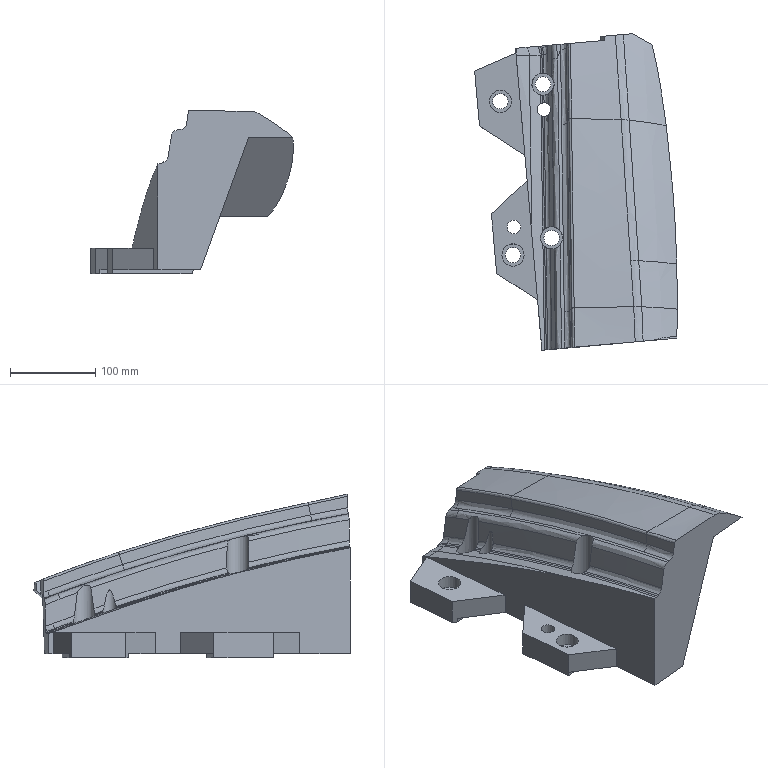Part | NX | features solid 2 | 1 solid | 92 faces | box 237.398 x 370.639 x 191.883 mm | volume 3889788 mm3 | spline 53 | plane 29 | cylinder 10 | commonest cylinder face diameters 18 x4 26 x4 16 x2